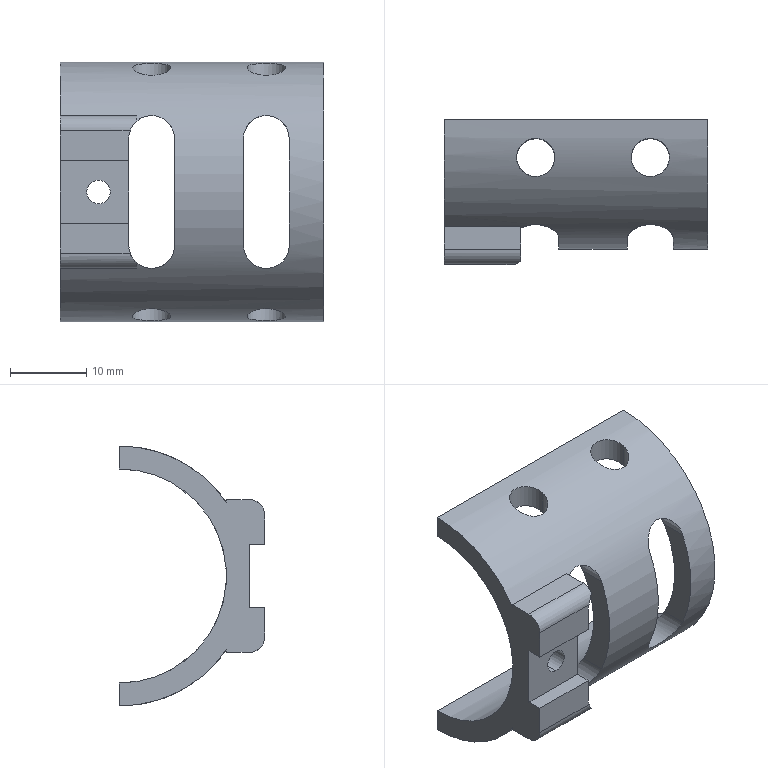Part | STEP file | Chain frame | 1 solid | 43 faces | box 34.45 x 19 x 34 mm | volume 4420 mm3 | cylinder 23 | plane 20 | commonest cylinder face diameters 5 x8 6 x6 8 x3 3.1 x2 4 x2 28 x1